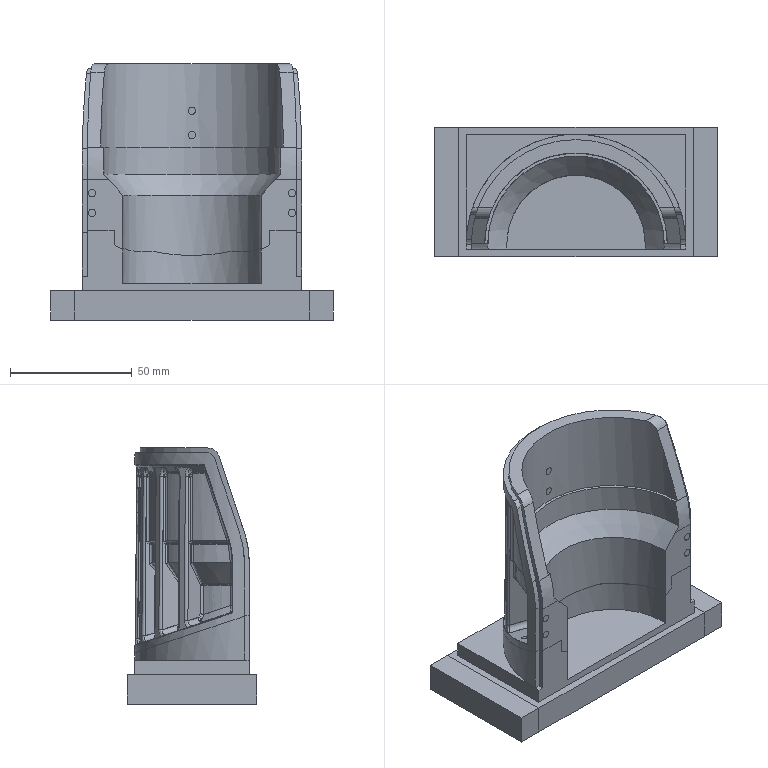NC program | NX | posted by the shop | part box 116 x 53 x 105 mm
Lines 61286 to 62366 of 572762:
T10 M6
;(T10:J-D2  D=2. R=0.)
;(XY=-0.03mm Z=-0.03mm)
G54 G90 D1
CYCLE832(0.04,_TOP_SURFACE_SMOOTH_ON+_ORI_SEMIFIN,1.)
CYCLE800(0,"AFMING",100000,57,0.,0.,0.,-90.,0.,-0.,0.,0.,0.,-1,100.,1)
G0 X0.0 Y29.209 S7000 M3 M8
Z58.55
X0.0 Y29.209 Z58.55
Z19.55
G1 X.027 Y29.071 F600.
X.127 Y28.971
X.265 Y28.944
X.402 Y28.971
X.503 Y29.071
X.53 Y29.209
X.462 Y29.489 Z19.541
X.249 Y29.688 Z19.533
X-.036 Y29.748 Z19.524
X-.31 Y29.651 Z19.515
X-.494 Y29.426 Z19.507
X-.535 Y29.138 Z19.4979
X-.421 Y28.871 Z19.489
X-.184 Y28.701 Z19.481
X.106 Y28.68 Z19.472
X.365 Y28.811 Z19.463
X.5186 Y29.059 Z19.454
X.521 Y29.35 Z19.446
X.373 Y29.6 Z19.437
X.116 Y29.736 Z19.428
X-.175 Y29.72 Z19.42
X-.414 Y29.555 Z19.411
X-.534 Y29.29 Z19.402
X-.498 Y29.001 Z19.394
X-.318 Y28.773 Z19.385
X-.045 Y28.671 Z19.376
X.24 Y28.725 Z19.368
X.456 Y28.92 Z19.359
X.54 Y29.199 Z19.35
X.467 Y29.4806 Z19.342
X.258 Y29.6833 Z19.333
X-.026 Y29.748 Z19.324
X-.302 Y29.6567 Z19.316
X-.49 Y29.435 Z19.307
X-.536 Y29.148 Z19.2982
X-.427 Y28.878 Z19.29
X-.193 Y28.705 Z19.281
X.096 Y28.6777 Z19.272
X.358 Y28.805 Z19.263
X.516 Y29.049 Z19.255
X.524 Y29.34 Z19.2461
X.38 Y29.593 Z19.237
X.125 Y29.734 Z19.229
X-.165 Y29.723 Z19.22
X-.408 Y29.563 Z19.211
X-.532 Y29.3 Z19.203
X-.502 Y29.01 Z19.194
X-.326 Y28.779 Z19.185
X-.055 Y28.6719 Z19.177
X.231 Y28.721 Z19.168
X.451 Y28.912 Z19.159
X.54 Y29.1891 Z19.151
X.472 Y29.472 Z19.1419
X.267 Y29.678 Z19.133
X-.0157 Y29.749 Z19.125
X-.293 Y29.662 Z19.116
X-.486 Y29.4441 Z19.107
X-.537 Y29.158 Z19.098
X-.433 Y28.8863 Z19.09
X-.203 Y28.709 Z19.081
X.086 Y28.676 Z19.072
X.35 Y28.798 Z19.064
X.513 Y29.04 Z19.055
X.5261 Y29.33 Z19.046
X.387 Y29.586 Z19.038
X.1351 Y29.732 Z19.029
X-.156 Y29.726 Z19.02
X-.401 Y29.57 Z19.012
X-.531 Y29.309 Z19.003
X-.506 Y29.0195 Z18.994
X-.334 Y28.785 Z18.986
X-.065 Y28.673 Z18.977
X.222 Y28.717 Z18.968
X.445 Y28.904 Z18.96
X.5391 Y29.179 Z18.951
X.4763 Y29.463 Z18.9422
X.275 Y29.673 Z18.934
X-.006 Y29.749 Z18.925
X-.285 Y29.6675 Z18.916
X-.482 Y29.453 Z18.907
X-.538 Y29.168 Z18.899
X-.439 Y28.894 Z18.8901
X-.212 Y28.712 Z18.881
X.077 Y28.675 Z18.873
X.343 Y28.792 Z18.864
X.51 Y29.03 Z18.855
X.528 Y29.321 Z18.847
X.394 Y29.579 Z18.838
X.145 Y29.729 Z18.829
X-.146 Y29.729 Z18.821
X-.3947 Y29.577 Z18.812
X-.529 Y29.3191 Z18.803
X-.509 Y29.029 Z18.795
X-.342 Y28.791 Z18.7859
X-.075 Y28.6743 Z18.777
X.213 Y28.713 Z18.769
X.44 Y28.896 Z18.76
X.538 Y29.169 Z18.751
X.4809 Y29.454 Z18.742
X.284 Y29.668 Z18.734
X.004 Y29.749 Z18.725
X-.277 Y29.673 Z18.716
X-.477 Y29.462 Z18.708
X-.539 Y29.178 Z18.699
X-.444 Y28.902 Z18.69
X-.2209 Y28.716 Z18.682
X.067 Y28.6732 Z18.673
X.335 Y28.786 Z18.664
X.506 Y29.021 Z18.656
X.53 Y29.311 Z18.647
X.4 Y29.571 Z18.638
X.154 Y29.726 Z18.63
X-.137 Y29.731 Z18.621
X-.388 Y29.585 Z18.612
X-.526 Y29.329 Z18.604
X-.512 Y29.038 Z18.595
X-.349 Y28.797 Z18.5862
X-.085 Y28.676 Z18.578
X.204 Y28.709 Z18.569
X.434 Y28.888 Z18.56
X.538 Y29.159 Z18.551
X.485 Y29.446 Z18.543
X.292 Y29.663 Z18.5341
X.014 Y29.749 Z18.525
X-.268 Y29.678 Z18.517
X-.472 Y29.471 Z18.508
X-.5395 Y29.188 Z18.499
X-.45 Y28.911 Z18.491
X-.23 Y28.72 Z18.482
X.057 Y28.672 Z18.473
X.327 Y28.78 Z18.465
X.5026 Y29.012 Z18.456
X.532 Y29.301 Z18.447
X.407 Y29.564 Z18.439
X.164 Y29.723 Z18.4299
X-.127 Y29.734 Z18.421
X-.381 Y29.592 Z18.413
X-.524 Y29.338 Z18.404
X-.515 Y29.048 Z18.395
X-.357 Y28.804 Z18.386
X-.095 Y28.677 Z18.378
X.195 Y28.705 Z18.369
X.428 Y28.88 Z18.36
X.537 Y29.149 Z18.352
X.49 Y29.437 Z18.343
X.3 Y29.658 Z18.334
X.024 Y29.748 Z18.326
X-.259 Y29.683 Z18.317
X-.467 Y29.479 Z18.308
X-.5398 Y29.197 Z18.3
X-.455 Y28.919 Z18.291
X-.239 Y28.725 Z18.282
X.047 Y28.6711 Z18.274
X.319 Y28.7736 Z18.265
X.499 Y29.002 Z18.256
X.5336 Y29.291 Z18.248
X.4134 Y29.556 Z18.239
X.173 Y29.72 Z18.2302
X-.117 Y29.736 Z18.222
X-.374 Y29.599 Z18.213
X-.522 Y29.3481 Z18.204
X-.518 Y29.0572 Z18.195
X-.364 Y28.81 Z18.187
X-.104 Y28.679 Z18.1781
X.186 Y28.702 Z18.169
X.422 Y28.872 Z18.161
X.535 Y29.1396 Z18.152
X.494 Y29.428 Z18.143
X.309 Y29.652 Z18.135
X.034 Y29.748 Z18.126
X-.251 Y29.687 Z18.117
X-.462 Y29.488 Z18.109
X-.54 Y29.207 Z18.1
X-.461 Y28.927 Z18.091
X-.248 Y28.729 Z18.083
X.037 Y28.67 Z18.0739
X.311 Y28.768 Z18.065
X.495 Y28.993 Z18.057
X.535 Y29.2815 Z18.048
X.42 Y29.5486 Z18.039
X.183 Y29.717 Z18.03
X-.1076 Y29.738 Z18.022
X-.367 Y29.605 Z18.013
X-.519 Y29.358 Z18.004
X-.521 Y29.067 Z17.996
X-.371 Y28.817 Z17.987
X-.114 Y28.681 Z17.978
X.1762 Y28.699 Z17.97
X.415 Y28.864 Z17.961
X.534 Y29.13 Z17.952
X.498 Y29.418 Z17.944
X.317 Y29.646 Z17.935
X.044 Y29.747 Z17.926
X-.242 Y29.692 Z17.918
X-.457 Y29.496 Z17.909
X-.54 Y29.217 Z17.9
X-.466 Y28.936 Z17.892
X-.257 Y28.734 Z17.883
X.027 Y28.67 Z17.8742
X.303 Y28.762 Z17.866
X.491 Y28.984 Z17.857
X.536 Y29.272 Z17.848
X.426 Y29.541 Z17.839
X.192 Y29.714 Z17.831
X-.098 Y29.74 Z17.8221
X-.359 Y29.6121 Z17.813
X-.516 Y29.367 Z17.805
X-.523 Y29.076 Z17.796
X-.3786 Y28.824 Z17.787
X-.1239 Y28.683 Z17.779
X.167 Y28.695 Z17.77
X.409 Y28.857 Z17.761
X.533 Y29.12 Z17.753
X.501 Y29.4092 Z17.744
X.325 Y29.64 Z17.735
X.054 Y29.746 Z17.727
X-.233 Y29.696 Z17.7179
X-.4518 Y29.5046 Z17.709
X-.54 Y29.227 Z17.701
X-.471 Y28.945 Z17.692
X-.265 Y28.739 Z17.683
X.017 Y28.669 Z17.674
X.295 Y28.757 Z17.666
X.487 Y28.975 Z17.657
X.537 Y29.262 Z17.648
X.432 Y29.533 Z17.64
X.201 Y29.71 Z17.631
X-.088 Y29.742 Z17.622
X-.352 Y29.619 Z17.614
X-.513 Y29.377 Z17.605
X-.526 Y29.086 Z17.596
X-.386 Y28.831 Z17.588
X-.134 Y28.686 Z17.579
X.157 Y28.692 Z17.5703
X.402 Y28.849 Z17.562
X.5308 Y29.11 Z17.553
X.505 Y29.4 Z17.544
X.333 Y29.634 Z17.536
X.064 Y29.745 Z17.527
X-.2238 Y29.7 Z17.5182
X-.446 Y29.513 Z17.51
X-.539 Y29.237 Z17.501
X-.476 Y28.9533 Z17.492
X-.274 Y28.744 Z17.483
X.007 Y28.6691 Z17.475
X.286 Y28.751 Z17.4661
X.482 Y28.966 Z17.457
X.538 Y29.252 Z17.449
X.438 Y29.525 Z17.44
X.21 Y29.706 Z17.431
X-.078 Y29.7432 Z17.423
X-.344 Y29.625 Z17.414
X-.51 Y29.3861 Z17.405
X-.528 Y29.096 Z17.397
X-.393 Y28.838 Z17.388
X-.143 Y28.688 Z17.379
X.148 Y28.69 Z17.371
X.396 Y28.842 Z17.362
X.529 Y29.1 Z17.353
X.508 Y29.391 Z17.345
X.34 Y29.628 Z17.336
X.074 Y29.744 Z17.327
X-.215 Y29.704 Z17.318
X-.441 Y29.521 Z17.31
X-.539 Y29.2471 Z17.301
X-.48 Y28.9621 Z17.292
X-.282 Y28.749 Z17.284
X-.003 Y28.669 Z17.275
X.278 Y28.7461 Z17.266
X.4778 Y28.958 Z17.258
X.539 Y29.242 Z17.249
X.444 Y29.517 Z17.24
X.219 Y29.702 Z17.232
X-.068 Y29.745 Z17.223
X-.336 Y29.631 Z17.2143
X-.5067 Y29.395 Z17.206
X-.53 Y29.105 Z17.197
X-.399 Y28.846 Z17.188
X-.153 Y28.6911 Z17.18
X.138 Y28.687 Z17.171
X.389 Y28.8345 Z17.1622
X.527 Y29.091 Z17.154
X.512 Y29.381 Z17.145
X.348 Y29.622 Z17.136
X.083 Y29.742 Z17.127
X-.206 Y29.708 Z17.119
X-.435 Y29.529 Z17.1101
X-.538 Y29.257 Z17.101
X-.485 Y28.971 Z17.093
X-.291 Y28.754 Z17.084
X-.013 Y28.6692 Z17.075
X.269 Y28.741 Z17.067
X.473 Y28.949 Z17.058
X.539 Y29.232 Z17.049
X.449 Y29.509 Z17.041
X.228 Y29.698 Z17.032
X-.059 Y29.746 Z17.023
X-.329 Y29.637 Z17.015
X-.503 Y29.405 Z17.006
X-.532 Y29.115 Z16.997
X-.406 Y28.853 Z16.989
X-.162 Y28.694 Z16.98
X.129 Y28.685 Z16.971
X.382 Y28.8274 Z16.962
X.525 Y29.081 Z16.954
X.515 Y29.372 Z16.945
X.356 Y29.615 Z16.936
X.093 Y29.7408 Z16.928
X-.196 Y29.712 Z16.919
X-.429 Y29.537 Z16.91
X-.537 Y29.267 Z16.902
X-.489 Y28.98 Z16.893
X-.299 Y28.759 Z16.884
X-.022 Y28.67 Z16.876
X.261 Y28.736 Z16.867
X.468 Y28.94 Z16.8583
X.54 Y29.2221 Z16.85
X.4546 Y29.5 Z16.841
X.237 Y29.694 Z16.832
X-.049 Y29.7467 Z16.824
X-.3206 Y29.6434 Z16.815
X-.499 Y29.414 Z16.8062
X-.533 Y29.125 Z16.798
X-.412 Y28.86 Z16.789
X-.172 Y28.697 Z16.78
X.119 Y28.6823 Z16.771
X.375 Y28.82 Z16.763
X.5221 Y29.071 Z16.7541
X.5177 Y29.362 Z16.745
X.363 Y29.609 Z16.737
X.103 Y29.739 Z16.728
X-.187 Y29.715 Z16.719
X-.423 Y29.545 Z16.711
X-.536 Y29.277 Z16.702
X-.493 Y28.989 Z16.693
X-.307 Y28.765 Z16.685
X-.032 Y28.67 Z16.676
X.252 Y28.731 Z16.667
X.463 Y28.932 Z16.659
X.54 Y29.212 Z16.65
X.46 Y29.492 Z16.641
X.246 Y29.689 Z16.633
X-.039 Y29.7475 Z16.624
X-.313 Y29.649 Z16.615
X-.496 Y29.423 Z16.606
X-.535 Y29.135 Z16.598
X-.419 Y28.868 Z16.589
X-.181 Y28.7 Z16.58
X.109 Y28.6802 Z16.572
X.3677 Y28.8136 Z16.563
X.519 Y29.0618 Z16.554
X.52 Y29.353 Z16.546
X.3703 Y29.6019 Z16.537
X.113 Y29.737 Z16.528
X-.1777 Y29.719 Z16.52
X-.416 Y29.553 Z16.511
X-.534 Y29.287 Z16.5023
X-.497 Y28.998 Z16.494
X-.315 Y28.771 Z16.485
X-.042 Y28.671 Z16.476
X.243 Y28.7269 Z16.468
X.458 Y28.923 Z16.459
X.54 Y29.202 Z16.4502
X.465 Y29.483 Z16.442
X.255 Y29.685 Z16.433
X-.029 Y29.748 Z16.424
X-.3044 Y29.655 Z16.415
X-.492 Y29.432 Z16.407
X-.536 Y29.145 Z16.3981
X-.425 Y28.876 Z16.389
X-.19 Y28.704 Z16.381
X.099 Y28.678 Z16.372
X.36 Y28.8069 Z16.363
X.517 Y29.052 Z16.355
X.523 Y29.343 Z16.346
X.377 Y29.595 Z16.337
X.122 Y29.735 Z16.329
X-.168 Y29.722 Z16.32
X-.41 Y29.5602 Z16.311
X-.533 Y29.296 Z16.303
X-.501 Y29.007 Z16.294
X-.323 Y28.777 Z16.285
X-.052 Y28.672 Z16.277
X.234 Y28.723 Z16.268
X.453 Y28.915 Z16.259
X.54 Y29.192 Z16.25
X.47 Y29.475 Z16.242
X.264 Y29.68 Z16.233
X-.019 Y29.749 Z16.224
X-.296 Y29.66 Z16.216
X-.487 Y29.441 Z16.207
X-.537 Y29.1546 Z16.198
X-.431 Y28.884 Z16.19
X-.2 Y28.707 Z16.181
X.09 Y28.677 Z16.172
X.3529 Y28.8 Z16.164
X.514 Y29.043 Z16.155
X.525 Y29.333 Z16.1463
X.385 Y29.588 Z16.138
X.132 Y29.733 Z16.129
X-.159 Y29.725 Z16.12
X-.404 Y29.568 Z16.112
X-.531 Y29.306 Z16.103
X-.504 Y29.017 Z16.0942
X-.331 Y28.783 Z16.086
X-.062 Y28.673 Z16.077
X.225 Y28.718 Z16.068
X.447 Y28.9064 Z16.059
X.539 Y29.182 Z16.051
X.475 Y29.466 Z16.0421
X.272 Y29.6751 Z16.033
X-.009 Y29.749 Z16.025
X-.288 Y29.666 Z16.016
X-.483 Y29.45 Z16.007
X-.538 Y29.164 Z15.999
X-.437 Y28.892 Z15.99
X-.209 Y28.711 Z15.981
X.08 Y28.675 Z15.973
X.345 Y28.794 Z15.964
X.511 Y29.033 Z15.955
X.528 Y29.324 Z15.947
X.391 Y29.581 Z15.938
X.142 Y29.73 Z15.929
X-.149 Y29.728 Z15.921
X-.397 Y29.575 Z15.912
X-.529 Y29.316 Z15.903
X-.508 Y29.026 Z15.894
X-.339 Y28.789 Z15.886
X-.072 Y28.674 Z15.877
X.216 Y28.714 Z15.868
X.442 Y28.898 Z15.86
X.539 Y29.172 Z15.851
X.479 Y29.457 Z15.842
X.281 Y29.67 Z15.834
X.001 Y29.749 Z15.825
X-.279 Y29.671 Z15.816
X-.479 Y29.459 Z15.808
X-.539 Y29.1744 Z15.799
X-.443 Y28.9 Z15.7903
X-.218 Y28.715 Z15.782
X.07 Y28.6736 Z15.773
X.338 Y28.788 Z15.764
X.507 Y29.024 Z15.756
X.5296 Y29.314 Z15.747
X.3982 Y29.5736 Z15.7382
X.151 Y29.7273 Z15.73
X-.14 Y29.7305 Z15.721
X-.39 Y29.5823 Z15.712
X-.527 Y29.3257 Z15.703
X-.5112 Y29.035 Z15.695
X-.347 Y28.795 Z15.6861
X-.082 Y28.675 Z15.677
X.207 Y28.71 Z15.669
X.436 Y28.89 Z15.66
X.538 Y29.163 Z15.651
X.484 Y29.4484 Z15.643
X.289 Y29.665 Z15.634
X.011 Y29.749 Z15.625
X-.271 Y29.676 Z15.617
X-.474 Y29.468 Z15.608
X-.539 Y29.184 Z15.599
X-.448 Y28.908 Z15.591
X-.227 Y28.719 Z15.582
X.06 Y28.672 Z15.573
X.33 Y28.781 Z15.565
X.504 Y29.015 Z15.556
X.531 Y29.304 Z15.547
X.405 Y29.566 Z15.538
X.1607 Y29.724 Z15.53
X-.1301 Y29.733 Z15.521
X-.383 Y29.589 Z15.512
X-.525 Y29.335 Z15.504
X-.514 Y29.045 Z15.495
X-.354 Y28.802 Z15.4864
X-.092 Y28.677 Z15.478
X.198 Y28.7066 Z15.469
X.43 Y28.882 Z15.46
X.537 Y29.153 Z15.452
X.488 Y29.439 Z15.443
X.298 Y29.659 Z15.4343
X.021 Y29.748 Z15.426
X-.262 Y29.681 Z15.417
X-.469 Y29.476 Z15.408
X-.54 Y29.194 Z15.4
X-.454 Y28.916 Z15.391
X-.236 Y28.723 Z15.3822
X.05 Y28.671 Z15.374
X.322 Y28.775 Z15.365
X.5 Y29.005 Z15.356
X.533 Y29.294 Z15.347
X.411 Y29.5587 Z15.339
X.17 Y29.721 Z15.3301
X-.12 Y29.735 Z15.321
X-.376 Y29.5964 Z15.313
X-.5225 Y29.345 Z15.304
X-.517 Y29.054 Z15.295
X-.362 Y28.808 Z15.287
X-.101 Y28.679 Z15.278
X.189 Y28.703 Z15.269
X.424 Y28.874 Z15.261
X.536 Y29.143 Z15.252
X.492 Y29.43 Z15.243
X.306 Y29.654 Z15.235
X.031 Y29.748 Z15.226
X-.2534 Y29.686 Z15.217
X-.464 Y29.485 Z15.209
X-.5399 Y29.204 Z15.2
X-.459 Y28.925 Z15.191
X-.245 Y28.728 Z15.182
X.04 Y28.671 Z15.174
X.314 Y28.77 Z15.165
X.496 Y28.996 Z15.156
X.535 Y29.285 Z15.148
X.418 Y29.551 Z15.139
X.18 Y29.718 Z15.1304
X-.111 Y29.737 Z15.122
X-.369 Y29.603 Z15.113
X-.52 Y29.355 Z15.104
X-.52 Y29.064 Z15.096
X-.369 Y28.815 Z15.087
X-.111 Y28.6806 Z15.0783
X.179 Y28.7 Z15.07
X.417 Y28.867 Z15.061
X.535 Y29.133 Z15.052
X.496 Y29.421 Z15.044
X.314 Y29.648 Z15.035
X.0407 Y29.747 Z15.0262
X-.245 Y29.69 Z15.018
X-.459 Y29.494 Z15.009
X-.5399 Y29.214 Z15.
X-.4642 Y28.933 Z14.991
X-.254 Y28.732 Z14.983
X.03 Y28.67 Z14.9741
X.306 Y28.764 Z14.965
X.492 Y28.987 Z14.957
X.536 Y29.275 Z14.948
X.424 Y29.543 Z14.939
X.1889 Y29.715 Z14.931
X-.101 Y29.739 Z14.922
X-.362 Y29.61 Z14.913
X-.517 Y29.364 Z14.905
X-.5226 Y29.073 Z14.896
X-.376 Y28.822 Z14.887
X-.1208 Y28.683 Z14.879
X.167 Y28.706 Z14.87
X.353 Y28.8
X.482 Y28.967
X.538 Y29.17
X.503 Y29.376
X.409 Y29.562
X.242 Y29.691
X.039 Y29.747
X-.167 Y29.712
X-.353 Y29.618
X-.482 Y29.451
X-.538 Y29.248
X-.503 Y29.042
X-.409 Y28.856
X-.242 Y28.726
X-.039 Y28.67
X.167 Y28.706
X.289 Y28.775
X.353 Y28.902
X.335 Y29.041
X.266 Y29.163
X.139 Y29.227
X0.0 Y29.209
G0 Z58.55
Y19.209
Z19.55
G1 X.027 Y19.071
X.127 Y18.971
X.265 Y18.944
X.402 Y18.971
X.503 Y19.071
X.53 Y19.209
X.462 Y19.489 Z19.541
X.249 Y19.688 Z19.533
X-.036 Y19.748 Z19.524
X-.31 Y19.651 Z19.515
X-.494 Y19.426 Z19.507
X-.535 Y19.138 Z19.4979
X-.421 Y18.871 Z19.489
X-.184 Y18.701 Z19.481
X.106 Y18.68 Z19.472
X.365 Y18.811 Z19.463
X.5186 Y19.059 Z19.454
X.521 Y19.35 Z19.446
X.373 Y19.6 Z19.437
X.116 Y19.736 Z19.428
X-.175 Y19.72 Z19.42
X-.414 Y19.555 Z19.411
X-.534 Y19.29 Z19.402
X-.498 Y19.001 Z19.394
X-.318 Y18.773 Z19.385
X-.045 Y18.671 Z19.376
X.24 Y18.725 Z19.368
X.456 Y18.92 Z19.359
X.54 Y19.199 Z19.35
X.467 Y19.4806 Z19.342
X.258 Y19.6833 Z19.333
X-.026 Y19.748 Z19.324
X-.302 Y19.6567 Z19.316
X-.49 Y19.435 Z19.307
X-.536 Y19.148 Z19.2982
X-.427 Y18.878 Z19.29
X-.193 Y18.705 Z19.281
X.096 Y18.6777 Z19.272
X.358 Y18.805 Z19.263
X.516 Y19.049 Z19.255
X.524 Y19.34 Z19.2461
X.38 Y19.593 Z19.237
X.125 Y19.734 Z19.229
X-.165 Y19.723 Z19.22
X-.408 Y19.563 Z19.211
X-.532 Y19.3 Z19.203
X-.502 Y19.01 Z19.194
X-.326 Y18.779 Z19.185
X-.055 Y18.6719 Z19.177
X.231 Y18.721 Z19.168
X.451 Y18.912 Z19.159
X.54 Y19.1891 Z19.151
X.472 Y19.472 Z19.1419
X.267 Y19.678 Z19.133
X-.0157 Y19.749 Z19.125
X-.293 Y19.662 Z19.116
X-.486 Y19.4441 Z19.107
X-.537 Y19.158 Z19.098
X-.433 Y18.8863 Z19.09
X-.203 Y18.709 Z19.081
X.086 Y18.676 Z19.072
X.35 Y18.798 Z19.064
X.513 Y19.04 Z19.055
X.5261 Y19.33 Z19.046
X.387 Y19.586 Z19.038
X.1351 Y19.732 Z19.029
X-.156 Y19.726 Z19.02
X-.401 Y19.57 Z19.012
X-.531 Y19.309 Z19.003
X-.506 Y19.0195 Z18.994
X-.334 Y18.785 Z18.986
X-.065 Y18.673 Z18.977
X.222 Y18.717 Z18.968
X.445 Y18.904 Z18.96
X.5391 Y19.179 Z18.951
X.4763 Y19.463 Z18.9422
X.275 Y19.673 Z18.934
X-.006 Y19.749 Z18.925
X-.285 Y19.6675 Z18.916
X-.482 Y19.453 Z18.907
X-.538 Y19.168 Z18.899
X-.439 Y18.894 Z18.8901
X-.212 Y18.712 Z18.881
X.077 Y18.675 Z18.873
X.343 Y18.792 Z18.864
X.51 Y19.03 Z18.855
X.528 Y19.321 Z18.847
X.394 Y19.579 Z18.838
X.145 Y19.729 Z18.829
X-.146 Y19.729 Z18.821
X-.3947 Y19.577 Z18.812
X-.529 Y19.3191 Z18.803
X-.509 Y19.029 Z18.795
X-.342 Y18.791 Z18.7859
X-.075 Y18.6743 Z18.777
X.213 Y18.713 Z18.769
X.44 Y18.896 Z18.76
X.538 Y19.169 Z18.751
X.4809 Y19.454 Z18.742
X.284 Y19.668 Z18.734
X.004 Y19.749 Z18.725
X-.277 Y19.673 Z18.716
X-.477 Y19.462 Z18.708
X-.539 Y19.178 Z18.699
X-.444 Y18.902 Z18.69
X-.2209 Y18.716 Z18.682
X.067 Y18.6732 Z18.673
X.335 Y18.786 Z18.664
X.506 Y19.021 Z18.656
X.53 Y19.311 Z18.647
X.4 Y19.571 Z18.638
X.154 Y19.726 Z18.63
X-.137 Y19.731 Z18.621
X-.388 Y19.585 Z18.612
X-.526 Y19.329 Z18.604
X-.512 Y19.038 Z18.595
X-.349 Y18.797 Z18.5862
X-.085 Y18.676 Z18.578
X.204 Y18.709 Z18.569
X.434 Y18.888 Z18.56
X.538 Y19.159 Z18.551
X.485 Y19.446 Z18.543
X.292 Y19.663 Z18.5341
X.014 Y19.749 Z18.525
X-.268 Y19.678 Z18.517
X-.472 Y19.471 Z18.508
X-.5395 Y19.188 Z18.499
X-.45 Y18.911 Z18.491
X-.23 Y18.72 Z18.482
X.057 Y18.672 Z18.473
X.327 Y18.78 Z18.465
X.5026 Y19.012 Z18.456
X.532 Y19.301 Z18.447
X.407 Y19.564 Z18.439
X.164 Y19.723 Z18.4299
X-.127 Y19.734 Z18.421
X-.381 Y19.592 Z18.413
X-.524 Y19.338 Z18.404
X-.515 Y19.048 Z18.395
X-.357 Y18.804 Z18.386
X-.095 Y18.677 Z18.378
X.195 Y18.705 Z18.369
X.428 Y18.88 Z18.36
X.537 Y19.149 Z18.352
X.49 Y19.437 Z18.343
X.3 Y19.658 Z18.334
X.024 Y19.748 Z18.326
X-.259 Y19.683 Z18.317
X-.467 Y19.479 Z18.308
X-.5398 Y19.197 Z18.3
X-.455 Y18.919 Z18.291
X-.239 Y18.725 Z18.282
X.047 Y18.6711 Z18.274
X.319 Y18.7736 Z18.265
X.499 Y19.002 Z18.256
X.5336 Y19.291 Z18.248
X.4134 Y19.556 Z18.239
X.173 Y19.72 Z18.2302
X-.117 Y19.736 Z18.222
X-.374 Y19.599 Z18.213
X-.522 Y19.3481 Z18.204
X-.518 Y19.0572 Z18.195
X-.364 Y18.81 Z18.187
X-.104 Y18.679 Z18.1781
X.186 Y18.702 Z18.169
X.422 Y18.872 Z18.161
X.535 Y19.1396 Z18.152
X.494 Y19.428 Z18.143
X.309 Y19.652 Z18.135
X.034 Y19.748 Z18.126
X-.251 Y19.687 Z18.117
X-.462 Y19.488 Z18.109
X-.54 Y19.207 Z18.1
X-.461 Y18.927 Z18.091
X-.248 Y18.729 Z18.083
X.037 Y18.67 Z18.0739
X.311 Y18.768 Z18.065
X.495 Y18.993 Z18.057
X.535 Y19.2815 Z18.048
X.42 Y19.5486 Z18.039
X.183 Y19.717 Z18.03
X-.1076 Y19.738 Z18.022
X-.367 Y19.605 Z18.013
X-.519 Y19.358 Z18.004
X-.521 Y19.067 Z17.996
X-.371 Y18.817 Z17.987
X-.114 Y18.681 Z17.978
X.1762 Y18.699 Z17.97
X.415 Y18.864 Z17.961
X.534 Y19.13 Z17.952
X.498 Y19.418 Z17.944
X.317 Y19.646 Z17.935
X.044 Y19.747 Z17.926
X-.242 Y19.692 Z17.918
X-.457 Y19.496 Z17.909
X-.54 Y19.217 Z17.9
X-.466 Y18.936 Z17.892
X-.257 Y18.734 Z17.883
X.027 Y18.67 Z17.8742
X.303 Y18.762 Z17.866
X.491 Y18.984 Z17.857
X.536 Y19.272 Z17.848
X.426 Y19.541 Z17.839
X.192 Y19.714 Z17.831
X-.098 Y19.74 Z17.8221
X-.359 Y19.6121 Z17.813
X-.516 Y19.367 Z17.805
X-.523 Y19.076 Z17.796
X-.3786 Y18.824 Z17.787
X-.1239 Y18.683 Z17.779
X.167 Y18.695 Z17.77
X.409 Y18.857 Z17.761
X.533 Y19.12 Z17.753
X.501 Y19.4092 Z17.744
X.325 Y19.64 Z17.735
X.054 Y19.746 Z17.727
X-.233 Y19.696 Z17.7179
X-.4518 Y19.5046 Z17.709
X-.54 Y19.227 Z17.701
X-.471 Y18.945 Z17.692
X-.265 Y18.739 Z17.683
X.017 Y18.669 Z17.674
X.295 Y18.757 Z17.666
X.487 Y18.975 Z17.657
X.537 Y19.262 Z17.648
X.432 Y19.533 Z17.64
X.201 Y19.71 Z17.631
X-.088 Y19.742 Z17.622
X-.352 Y19.619 Z17.614
X-.513 Y19.377 Z17.605
X-.526 Y19.086 Z17.596
X-.386 Y18.831 Z17.588
X-.134 Y18.686 Z17.579
X.157 Y18.692 Z17.5703
X.402 Y18.849 Z17.562
X.5308 Y19.11 Z17.553
X.505 Y19.4 Z17.544
X.333 Y19.634 Z17.536
X.064 Y19.745 Z17.527
X-.2238 Y19.7 Z17.5182
X-.446 Y19.513 Z17.51
X-.539 Y19.237 Z17.501
X-.476 Y18.9533 Z17.492
X-.274 Y18.744 Z17.483
X.007 Y18.6691 Z17.475
X.286 Y18.751 Z17.4661
X.482 Y18.966 Z17.457
X.538 Y19.252 Z17.449
X.438 Y19.525 Z17.44
X.21 Y19.706 Z17.431
X-.078 Y19.7432 Z17.423
X-.344 Y19.625 Z17.414
X-.51 Y19.3861 Z17.405
X-.528 Y19.096 Z17.397
X-.393 Y18.838 Z17.388
X-.143 Y18.688 Z17.379
X.148 Y18.69 Z17.371
X.396 Y18.842 Z17.362
X.529 Y19.1 Z17.353
X.508 Y19.391 Z17.345
X.34 Y19.628 Z17.336
X.074 Y19.744 Z17.327
X-.215 Y19.704 Z17.318
X-.441 Y19.521 Z17.31
X-.539 Y19.2471 Z17.301
X-.48 Y18.9621 Z17.292
X-.282 Y18.749 Z17.284
X-.003 Y18.669 Z17.275
X.278 Y18.7461 Z17.266
X.4778 Y18.958 Z17.258
X.539 Y19.242 Z17.249
X.444 Y19.517 Z17.24
X.219 Y19.702 Z17.232
X-.068 Y19.745 Z17.223
X-.336 Y19.631 Z17.2143
X-.5067 Y19.395 Z17.206
X-.53 Y19.105 Z17.197
X-.399 Y18.846 Z17.188
X-.153 Y18.6911 Z17.18
X.138 Y18.687 Z17.171
X.389 Y18.8345 Z17.1622
X.527 Y19.091 Z17.154
X.512 Y19.381 Z17.145
X.348 Y19.622 Z17.136
X.083 Y19.742 Z17.127
X-.206 Y19.708 Z17.119
X-.435 Y19.529 Z17.1101
X-.538 Y19.257 Z17.101
X-.485 Y18.971 Z17.093
X-.291 Y18.754 Z17.084
X-.013 Y18.6692 Z17.075
X.269 Y18.741 Z17.067
X.473 Y18.949 Z17.058
X.539 Y19.232 Z17.049
X.449 Y19.509 Z17.041
X.228 Y19.698 Z17.032
X-.059 Y19.746 Z17.023
X-.329 Y19.637 Z17.015
X-.503 Y19.405 Z17.006
X-.532 Y19.115 Z16.997
X-.406 Y18.853 Z16.989
X-.162 Y18.694 Z16.98
X.129 Y18.685 Z16.971
X.382 Y18.8274 Z16.962
X.525 Y19.081 Z16.954
X.515 Y19.372 Z16.945
X.356 Y19.615 Z16.936
X.093 Y19.7408 Z16.928
X-.196 Y19.712 Z16.919
X-.429 Y19.537 Z16.91
X-.537 Y19.267 Z16.902
X-.489 Y18.98 Z16.893
X-.299 Y18.759 Z16.884
X-.022 Y18.67 Z16.876
X.261 Y18.736 Z16.867
X.468 Y18.94 Z16.8583
X.54 Y19.2221 Z16.85
X.4546 Y19.5 Z16.841
X.237 Y19.694 Z16.832
X-.049 Y19.7467 Z16.824
X-.3206 Y19.6434 Z16.815
X-.499 Y19.414 Z16.8062
X-.533 Y19.125 Z16.798
X-.412 Y18.86 Z16.789
X-.172 Y18.697 Z16.78
X.119 Y18.6823 Z16.771
X.375 Y18.82 Z16.763
X.5221 Y19.071 Z16.7541
X.5177 Y19.362 Z16.745
X.363 Y19.609 Z16.737
X.103 Y19.739 Z16.728
X-.187 Y19.715 Z16.719
X-.423 Y19.545 Z16.711
X-.536 Y19.277 Z16.702
X-.493 Y18.989 Z16.693
X-.307 Y18.765 Z16.685
X-.032 Y18.67 Z16.676
X.252 Y18.731 Z16.667
X.463 Y18.932 Z16.659
X.54 Y19.212 Z16.65
X.46 Y19.492 Z16.641
X.246 Y19.689 Z16.633
X-.039 Y19.7475 Z16.624
X-.313 Y19.649 Z16.615
X-.496 Y19.423 Z16.606
X-.535 Y19.135 Z16.598
X-.419 Y18.868 Z16.589
X-.181 Y18.7 Z16.58
X.109 Y18.6802 Z16.572
X.3677 Y18.8136 Z16.563
X.519 Y19.0618 Z16.554
X.52 Y19.353 Z16.546
X.3703 Y19.6019 Z16.537
X.113 Y19.737 Z16.528
X-.1777 Y19.719 Z16.52
X-.416 Y19.553 Z16.511
X-.534 Y19.287 Z16.5023
X-.497 Y18.998 Z16.494
X-.315 Y18.771 Z16.485
X-.042 Y18.671 Z16.476
X.243 Y18.7269 Z16.468
X.458 Y18.923 Z16.459
X.54 Y19.202 Z16.4502
X.465 Y19.483 Z16.442
X.255 Y19.685 Z16.433
X-.029 Y19.748 Z16.424
X-.3044 Y19.655 Z16.415
X-.492 Y19.432 Z16.407
X-.536 Y19.145 Z16.3981
X-.425 Y18.876 Z16.389
X-.19 Y18.704 Z16.381
X.099 Y18.678 Z16.372
X.36 Y18.8069 Z16.363
X.517 Y19.052 Z16.355
X.523 Y19.343 Z16.346
X.377 Y19.595 Z16.337
X.122 Y19.735 Z16.329
X-.168 Y19.722 Z16.32
X-.41 Y19.5602 Z16.311
X-.533 Y19.296 Z16.303
X-.501 Y19.007 Z16.294
X-.323 Y18.777 Z16.285
X-.052 Y18.672 Z16.277
X.234 Y18.723 Z16.268
X.453 Y18.915 Z16.259
X.54 Y19.192 Z16.25
X.47 Y19.475 Z16.242
X.264 Y19.68 Z16.233
X-.019 Y19.749 Z16.224
X-.296 Y19.66 Z16.216
X-.487 Y19.441 Z16.207
X-.537 Y19.1546 Z16.198
X-.431 Y18.884 Z16.19
X-.2 Y18.707 Z16.181
X.09 Y18.677 Z16.172
X.3529 Y18.8 Z16.164
X.514 Y19.043 Z16.155
X.525 Y19.333 Z16.1463
X.385 Y19.588 Z16.138
X.132 Y19.733 Z16.129
X-.159 Y19.725 Z16.12
X-.404 Y19.568 Z16.112
X-.531 Y19.306 Z16.103
X-.504 Y19.017 Z16.0942
X-.331 Y18.783 Z16.086
X-.062 Y18.673 Z16.077
X.225 Y18.718 Z16.068
X.447 Y18.9064 Z16.059
X.539 Y19.182 Z16.051
X.475 Y19.466 Z16.0421
X.272 Y19.6751 Z16.033
X-.009 Y19.749 Z16.025
X-.288 Y19.666 Z16.016
X-.483 Y19.45 Z16.007
X-.538 Y19.164 Z15.999
X-.437 Y18.892 Z15.99
X-.209 Y18.711 Z15.981
X.08 Y18.675 Z15.973
X.345 Y18.794 Z15.964
X.511 Y19.033 Z15.955
X.528 Y19.324 Z15.947
X.391 Y19.581 Z15.938
X.142 Y19.73 Z15.929
X-.149 Y19.728 Z15.921
X-.397 Y19.575 Z15.912
X-.529 Y19.316 Z15.903
X-.508 Y19.026 Z15.894
X-.339 Y18.789 Z15.886
X-.072 Y18.674 Z15.877
X.216 Y18.714 Z15.868
X.442 Y18.898 Z15.86
X.539 Y19.172 Z15.851
X.479 Y19.457 Z15.842
X.281 Y19.67 Z15.834
X.001 Y19.749 Z15.825
X-.279 Y19.671 Z15.816
X-.479 Y19.459 Z15.808
X-.539 Y19.1744 Z15.799
X-.443 Y18.9 Z15.7903
X-.218 Y18.715 Z15.782
X.07 Y18.6736 Z15.773
X.338 Y18.788 Z15.764
X.507 Y19.024 Z15.756
X.5296 Y19.314 Z15.747
X.3982 Y19.5736 Z15.7382
X.151 Y19.7273 Z15.73
X-.14 Y19.7305 Z15.721
X-.39 Y19.5823 Z15.712
X-.527 Y19.3257 Z15.703
X-.5112 Y19.035 Z15.695
X-.347 Y18.795 Z15.6861
X-.082 Y18.675 Z15.677
X.207 Y18.71 Z15.669
X.436 Y18.89 Z15.66
X.538 Y19.163 Z15.651
X.484 Y19.4484 Z15.643
X.289 Y19.665 Z15.634
X.011 Y19.749 Z15.625
X-.271 Y19.676 Z15.617
X-.474 Y19.468 Z15.608
X-.539 Y19.184 Z15.599
X-.448 Y18.908 Z15.591
X-.227 Y18.719 Z15.582
X.06 Y18.672 Z15.573
X.33 Y18.781 Z15.565
X.504 Y19.015 Z15.556
X.531 Y19.304 Z15.547
X.405 Y19.566 Z15.538
X.1607 Y19.724 Z15.53
X-.1301 Y19.733 Z15.521
X-.383 Y19.589 Z15.512
X-.525 Y19.335 Z15.504
X-.514 Y19.045 Z15.495
X-.354 Y18.802 Z15.4864
X-.092 Y18.677 Z15.478
X.198 Y18.7066 Z15.469
X.43 Y18.882 Z15.46
X.537 Y19.153 Z15.452
X.488 Y19.439 Z15.443
X.298 Y19.659 Z15.4343
X.021 Y19.748 Z15.426
X-.262 Y19.681 Z15.417
X-.469 Y19.476 Z15.408
X-.54 Y19.194 Z15.4
X-.454 Y18.916 Z15.391
X-.236 Y18.723 Z15.3822
X.05 Y18.671 Z15.374
X.322 Y18.775 Z15.365
X.5 Y19.005 Z15.356
X.533 Y19.294 Z15.347
X.411 Y19.5587 Z15.339
X.17 Y19.721 Z15.3301
X-.12 Y19.735 Z15.321
X-.376 Y19.5964 Z15.313
X-.5225 Y19.345 Z15.304
X-.517 Y19.054 Z15.295
X-.362 Y18.808 Z15.287
X-.101 Y18.679 Z15.278
X.189 Y18.703 Z15.269
X.424 Y18.874 Z15.261
X.536 Y19.143 Z15.252